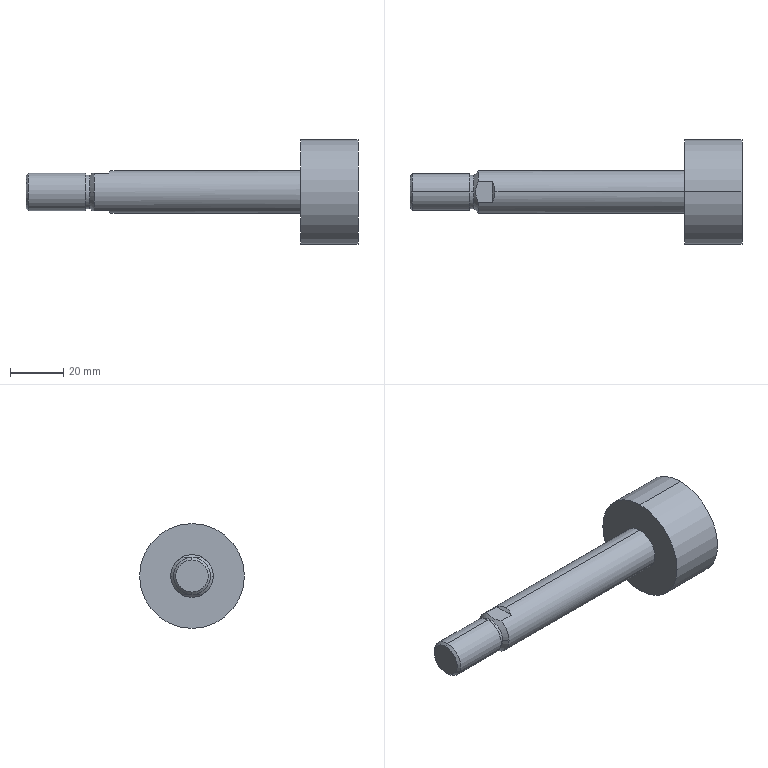Part | SolidWorks | features BaseBody 1 | 1 solid | 20 faces | box 125 x 39.5 x 39.5 mm | volume 45935 mm3 | cylinder 8 | plane 8 | cone 4 | commonest cylinder face diameters 12.6 x2 14 x2 16 x2 39.5 x2
STEP:
#1=CARTESIAN_POINT('',(-19.,3.873,7.));
#2=VERTEX_POINT('',#1);
#3=CARTESIAN_POINT('',(-18.,0.,8.));
#4=VERTEX_POINT('',#3);
#5=CARTESIAN_POINT('',(-19.,3.873,7.));
#6=CARTESIAN_POINT('',(-18.341,2.681,7.659));
#7=CARTESIAN_POINT('',(-18.,1.362,8.));
#8=CARTESIAN_POINT('',(-18.,0.,8.));
#9=(BOUNDED_CURVE()B_SPLINE_CURVE(3,(#5,#6,#7,#8),.UNSPECIFIED.,.F.,.F.)B_SPLINE_CURVE_WITH_KNOTS((4,4),(5.778,6.283),.UNSPECIFIED.)CURVE()GEOMETRIC_REPRESENTATION_ITEM()RATIONAL_B_SPLINE_CURVE((1.,0.9788,0.9788,1.))REPRESENTATION_ITEM(''));
#10=EDGE_CURVE('',#2,#4,#9,.T.);
#11=ORIENTED_EDGE('',*,*,#10,.T.);
#12=CARTESIAN_POINT('',(53.4,0.,8.));
#13=VERTEX_POINT('',#12);
#14=CARTESIAN_POINT('',(75.,0.,8.));
#15=DIRECTION('',(1.,0.,0.));
#16=VECTOR('',#15,1000.);
#17=LINE('',#14,#16);
#18=EDGE_CURVE('',#4,#13,#17,.T.);
#19=ORIENTED_EDGE('',*,*,#18,.T.);
#20=CARTESIAN_POINT('',(53.4,0.,-8.));
#21=VERTEX_POINT('',#20);
#22=CARTESIAN_POINT('',(53.4,0.,0.));
#23=DIRECTION('',(-1.,0.,0.));
#24=DIRECTION('',(0.,0.,-1.));
#25=AXIS2_PLACEMENT_3D('',#22,#23,#24);
#26=CIRCLE('',#25,8.);
#27=EDGE_CURVE('',#13,#21,#26,.T.);
#28=ORIENTED_EDGE('',*,*,#27,.T.);
#29=CARTESIAN_POINT('',(-18.,0.,-8.));
#30=VERTEX_POINT('',#29);
#31=CARTESIAN_POINT('',(75.,0.,-8.));
#32=DIRECTION('',(1.,0.,0.));
#33=VECTOR('',#32,1000.);
#34=LINE('',#31,#33);
#35=EDGE_CURVE('',#30,#21,#34,.T.);
#36=ORIENTED_EDGE('',*,*,#35,.F.);
#37=CARTESIAN_POINT('',(-19.,3.873,-7.));
#38=VERTEX_POINT('',#37);
#39=CARTESIAN_POINT('',(-18.,0.,-8.));
#40=CARTESIAN_POINT('',(-18.,1.362,-8.));
#41=CARTESIAN_POINT('',(-18.341,2.681,-7.659));
#42=CARTESIAN_POINT('',(-19.,3.873,-7.));
#43=(BOUNDED_CURVE()B_SPLINE_CURVE(3,(#39,#40,#41,#42),.UNSPECIFIED.,.F.,.F.)B_SPLINE_CURVE_WITH_KNOTS((4,4),(0.,0.5054),.UNSPECIFIED.)CURVE()GEOMETRIC_REPRESENTATION_ITEM()RATIONAL_B_SPLINE_CURVE((1.,0.9788,0.9788,1.))REPRESENTATION_ITEM(''));
#44=EDGE_CURVE('',#30,#38,#43,.T.);
#45=ORIENTED_EDGE('',*,*,#44,.T.);
#46=CARTESIAN_POINT('',(-24.3,3.873,-7.));
#47=VERTEX_POINT('',#46);
#48=CARTESIAN_POINT('',(75.,3.873,-7.));
#49=DIRECTION('',(-1.,0.,0.));
#50=VECTOR('',#49,1000.);
#51=LINE('',#48,#50);
#52=EDGE_CURVE('',#38,#47,#51,.T.);
#53=ORIENTED_EDGE('',*,*,#52,.T.);
#54=CARTESIAN_POINT('',(-24.3,8.,0.));
#55=VERTEX_POINT('',#54);
#56=CARTESIAN_POINT('',(-24.3,0.,0.));
#57=DIRECTION('',(1.,0.,0.));
#58=DIRECTION('',(0.,0.,-1.));
#59=AXIS2_PLACEMENT_3D('',#56,#57,#58);
#60=CIRCLE('',#59,8.);
#61=EDGE_CURVE('',#47,#55,#60,.T.);
#62=ORIENTED_EDGE('',*,*,#61,.T.);
#63=CARTESIAN_POINT('',(-24.3,3.873,7.));
#64=VERTEX_POINT('',#63);
#65=CARTESIAN_POINT('',(-24.3,0.,0.));
#66=DIRECTION('',(1.,0.,0.));
#67=DIRECTION('',(0.,0.,-1.));
#68=AXIS2_PLACEMENT_3D('',#65,#66,#67);
#69=CIRCLE('',#68,8.);
#70=EDGE_CURVE('',#55,#64,#69,.T.);
#71=ORIENTED_EDGE('',*,*,#70,.T.);
#72=CARTESIAN_POINT('',(75.,3.873,7.));
#73=DIRECTION('',(1.,0.,0.));
#74=VECTOR('',#73,1000.);
#75=LINE('',#72,#74);
#76=EDGE_CURVE('',#64,#2,#75,.T.);
#77=ORIENTED_EDGE('',*,*,#76,.T.);
#78=EDGE_LOOP('',(#11,#19,#28,#36,#45,#53,#62,#71,#77));
#79=FACE_OUTER_BOUND('',#78,.T.);
#80=CARTESIAN_POINT('',(75.,0.,0.));
#81=DIRECTION('',(1.,0.,0.));
#82=DIRECTION('',(0.,0.,-1.));
#83=AXIS2_PLACEMENT_3D('',#80,#81,#82);
#84=CYLINDRICAL_SURFACE('',#83,8.);
#85=ADVANCED_FACE('',(#79),#84,.T.);
#86=CARTESIAN_POINT('',(-26.,0.,6.3));
#87=VERTEX_POINT('',#86);
#88=CARTESIAN_POINT('',(-26.,-6.3,0.));
#89=VERTEX_POINT('',#88);
#90=CARTESIAN_POINT('',(-26.,0.,0.));
#91=DIRECTION('',(1.,0.,0.));
#92=DIRECTION('',(0.,0.,-1.));
#93=AXIS2_PLACEMENT_3D('',#90,#91,#92);
#94=CIRCLE('',#93,6.3);
#95=EDGE_CURVE('',#87,#89,#94,.T.);
#96=ORIENTED_EDGE('',*,*,#95,.T.);
#97=CARTESIAN_POINT('',(-24.3,-8.,0.));
#98=VERTEX_POINT('',#97);
#99=CARTESIAN_POINT('',(-24.3,-8.,0.));
#100=DIRECTION('',(0.7071,-0.7071,0.));
#101=VECTOR('',#100,1000.);
#102=LINE('',#99,#101);
#103=EDGE_CURVE('',#89,#98,#102,.T.);
#104=ORIENTED_EDGE('',*,*,#103,.T.);
#105=CARTESIAN_POINT('',(-24.3,-3.873,7.));
#106=VERTEX_POINT('',#105);
#107=CARTESIAN_POINT('',(-24.3,0.,0.));
#108=DIRECTION('',(1.,0.,0.));
#109=DIRECTION('',(0.,0.,-1.));
#110=AXIS2_PLACEMENT_3D('',#107,#108,#109);
#111=CIRCLE('',#110,8.);
#112=EDGE_CURVE('',#106,#98,#111,.T.);
#113=ORIENTED_EDGE('',*,*,#112,.F.);
#114=CARTESIAN_POINT('',(-24.3,3.873,7.));
#115=CARTESIAN_POINT('',(-24.594,3.265,7.));
#116=CARTESIAN_POINT('',(-24.843,2.645,7.));
#117=CARTESIAN_POINT('',(-25.107,1.682,7.));
#118=CARTESIAN_POINT('',(-25.177,1.356,7.));
#119=CARTESIAN_POINT('',(-25.274,0.6915,7.));
#120=CARTESIAN_POINT('',(-25.299,0.3497,7.));
#121=CARTESIAN_POINT('',(-25.301,-0.6617,7.));
#122=CARTESIAN_POINT('',(-25.204,-1.325,7.));
#123=CARTESIAN_POINT('',(-24.937,-2.305,7.));
#124=CARTESIAN_POINT('',(-24.829,-2.627,7.));
#125=CARTESIAN_POINT('',(-24.584,-3.258,7.));
#126=CARTESIAN_POINT('',(-24.448,-3.568,7.));
#127=CARTESIAN_POINT('',(-24.3,-3.873,7.));
#128=B_SPLINE_CURVE_WITH_KNOTS('',3,(#114,#115,#116,#117,#118,#119,#120,#121,#122,#123,#124,#125,#126,#127),.UNSPECIFIED.,.F.,.F.,(4,2,2,2,2,2,4),(0.,0.001996,0.002994,0.003992,0.005988,0.006986,0.007984),.UNSPECIFIED.);
#129=EDGE_CURVE('',#64,#106,#128,.T.);
#130=ORIENTED_EDGE('',*,*,#129,.F.);
#131=ORIENTED_EDGE('',*,*,#70,.F.);
#132=CARTESIAN_POINT('',(-26.,6.3,0.));
#133=VERTEX_POINT('',#132);
#134=CARTESIAN_POINT('',(-24.3,8.,0.));
#135=DIRECTION('',(0.7071,0.7071,0.));
#136=VECTOR('',#135,1000.);
#137=LINE('',#134,#136);
#138=EDGE_CURVE('',#133,#55,#137,.T.);
#139=ORIENTED_EDGE('',*,*,#138,.F.);
#140=CARTESIAN_POINT('',(-26.,0.,0.));
#141=DIRECTION('',(1.,0.,0.));
#142=DIRECTION('',(0.,0.,-1.));
#143=AXIS2_PLACEMENT_3D('',#140,#141,#142);
#144=CIRCLE('',#143,6.3);
#145=EDGE_CURVE('',#133,#87,#144,.T.);
#146=ORIENTED_EDGE('',*,*,#145,.T.);
#147=EDGE_LOOP('',(#96,#104,#113,#130,#131,#139,#146));
#148=FACE_OUTER_BOUND('',#147,.T.);
#149=CARTESIAN_POINT('',(-24.3,0.,0.));
#150=DIRECTION('',(1.,0.,0.));
#151=DIRECTION('',(0.,1.,0.));
#152=AXIS2_PLACEMENT_3D('',#149,#150,#151);
#153=CONICAL_SURFACE('',#152,8.,0.7854);
#154=ADVANCED_FACE('',(#148),#153,.T.);
#155=CARTESIAN_POINT('',(-27.5,0.,-6.3));
#156=VERTEX_POINT('',#155);
#157=CARTESIAN_POINT('',(-27.5,0.,6.3));
#158=VERTEX_POINT('',#157);
#159=CARTESIAN_POINT('',(-27.5,0.,0.));
#160=DIRECTION('',(1.,0.,0.));
#161=DIRECTION('',(0.,0.,-1.));
#162=AXIS2_PLACEMENT_3D('',#159,#160,#161);
#163=CIRCLE('',#162,6.3);
#164=EDGE_CURVE('',#156,#158,#163,.T.);
#165=ORIENTED_EDGE('',*,*,#164,.T.);
#166=CARTESIAN_POINT('',(75.,0.,6.3));
#167=DIRECTION('',(1.,0.,0.));
#168=VECTOR('',#167,1000.);
#169=LINE('',#166,#168);
#170=EDGE_CURVE('',#158,#87,#169,.T.);
#171=ORIENTED_EDGE('',*,*,#170,.T.);
#172=ORIENTED_EDGE('',*,*,#145,.F.);
#173=CARTESIAN_POINT('',(-26.,0.,-6.3));
#174=VERTEX_POINT('',#173);
#175=CARTESIAN_POINT('',(-26.,0.,0.));
#176=DIRECTION('',(1.,0.,0.));
#177=DIRECTION('',(0.,0.,-1.));
#178=AXIS2_PLACEMENT_3D('',#175,#176,#177);
#179=CIRCLE('',#178,6.3);
#180=EDGE_CURVE('',#174,#133,#179,.T.);
#181=ORIENTED_EDGE('',*,*,#180,.F.);
#182=CARTESIAN_POINT('',(75.,0.,-6.3));
#183=DIRECTION('',(1.,0.,0.));
#184=VECTOR('',#183,1000.);
#185=LINE('',#182,#184);
#186=EDGE_CURVE('',#156,#174,#185,.T.);
#187=ORIENTED_EDGE('',*,*,#186,.F.);
#188=EDGE_LOOP('',(#165,#171,#172,#181,#187));
#189=FACE_OUTER_BOUND('',#188,.T.);
#190=CARTESIAN_POINT('',(75.,0.,0.));
#191=DIRECTION('',(1.,0.,0.));
#192=DIRECTION('',(0.,0.,-1.));
#193=AXIS2_PLACEMENT_3D('',#190,#191,#192);
#194=CYLINDRICAL_SURFACE('',#193,6.3);
#195=ADVANCED_FACE('',(#189),#194,.T.);
#196=CARTESIAN_POINT('',(53.4,0.,-19.75));
#197=VERTEX_POINT('',#196);
#198=CARTESIAN_POINT('',(53.4,0.,19.75));
#199=VERTEX_POINT('',#198);
#200=CARTESIAN_POINT('',(53.4,0.,0.));
#201=DIRECTION('',(1.,0.,0.));
#202=DIRECTION('',(0.,0.,-1.));
#203=AXIS2_PLACEMENT_3D('',#200,#201,#202);
#204=CIRCLE('',#203,19.75);
#205=EDGE_CURVE('',#197,#199,#204,.T.);
#206=ORIENTED_EDGE('',*,*,#205,.T.);
#207=CARTESIAN_POINT('',(75.,0.,19.75));
#208=VERTEX_POINT('',#207);
#209=CARTESIAN_POINT('',(75.,0.,19.75));
#210=DIRECTION('',(1.,0.,0.));
#211=VECTOR('',#210,1000.);
#212=LINE('',#209,#211);
#213=EDGE_CURVE('',#199,#208,#212,.T.);
#214=ORIENTED_EDGE('',*,*,#213,.T.);
#215=CARTESIAN_POINT('',(75.,0.,-19.75));
#216=VERTEX_POINT('',#215);
#217=CARTESIAN_POINT('',(75.,0.,0.));
#218=DIRECTION('',(-1.,0.,0.));
#219=DIRECTION('',(0.,0.,-1.));
#220=AXIS2_PLACEMENT_3D('',#217,#218,#219);
#221=CIRCLE('',#220,19.75);
#222=EDGE_CURVE('',#208,#216,#221,.T.);
#223=ORIENTED_EDGE('',*,*,#222,.T.);
#224=CARTESIAN_POINT('',(75.,0.,-19.75));
#225=DIRECTION('',(1.,0.,0.));
#226=VECTOR('',#225,1000.);
#227=LINE('',#224,#226);
#228=EDGE_CURVE('',#197,#216,#227,.T.);
#229=ORIENTED_EDGE('',*,*,#228,.F.);
#230=EDGE_LOOP('',(#206,#214,#223,#229));
#231=FACE_OUTER_BOUND('',#230,.T.);
#232=CARTESIAN_POINT('',(75.,0.,0.));
#233=DIRECTION('',(1.,0.,0.));
#234=DIRECTION('',(0.,0.,-1.));
#235=AXIS2_PLACEMENT_3D('',#232,#233,#234);
#236=CYLINDRICAL_SURFACE('',#235,19.75);
#237=ADVANCED_FACE('',(#231),#236,.T.);
#238=CARTESIAN_POINT('',(-49.08,0.,-7.));
#239=VERTEX_POINT('',#238);
#240=CARTESIAN_POINT('',(-49.08,0.,7.));
#241=VERTEX_POINT('',#240);
#242=CARTESIAN_POINT('',(-49.08,0.,0.));
#243=DIRECTION('',(1.,0.,0.));
#244=DIRECTION('',(0.,0.,-1.));
#245=AXIS2_PLACEMENT_3D('',#242,#243,#244);
#246=CIRCLE('',#245,7.);
#247=EDGE_CURVE('',#239,#241,#246,.T.);
#248=ORIENTED_EDGE('',*,*,#247,.T.);
#249=CARTESIAN_POINT('',(-27.5,0.,7.));
#250=VERTEX_POINT('',#249);
#251=CARTESIAN_POINT('',(75.,0.,7.));
#252=DIRECTION('',(1.,0.,0.));
#253=VECTOR('',#252,1000.);
#254=LINE('',#251,#253);
#255=EDGE_CURVE('',#241,#250,#254,.T.);
#256=ORIENTED_EDGE('',*,*,#255,.T.);
#257=CARTESIAN_POINT('',(-27.5,0.,-7.));
#258=VERTEX_POINT('',#257);
#259=CARTESIAN_POINT('',(-27.5,0.,0.));
#260=DIRECTION('',(-1.,0.,0.));
#261=DIRECTION('',(0.,0.,-1.));
#262=AXIS2_PLACEMENT_3D('',#259,#260,#261);
#263=CIRCLE('',#262,7.);
#264=EDGE_CURVE('',#250,#258,#263,.T.);
#265=ORIENTED_EDGE('',*,*,#264,.T.);
#266=CARTESIAN_POINT('',(75.,0.,-7.));
#267=DIRECTION('',(1.,0.,0.));
#268=VECTOR('',#267,1000.);
#269=LINE('',#266,#268);
#270=EDGE_CURVE('',#239,#258,#269,.T.);
#271=ORIENTED_EDGE('',*,*,#270,.F.);
#272=EDGE_LOOP('',(#248,#256,#265,#271));
#273=FACE_OUTER_BOUND('',#272,.T.);
#274=CARTESIAN_POINT('',(75.,0.,0.));
#275=DIRECTION('',(1.,0.,0.));
#276=DIRECTION('',(0.,0.,-1.));
#277=AXIS2_PLACEMENT_3D('',#274,#275,#276);
#278=CYLINDRICAL_SURFACE('',#277,7.);
#279=ADVANCED_FACE('',(#273),#278,.T.);
#280=CARTESIAN_POINT('',(-50.,0.,-6.08));
#281=VERTEX_POINT('',#280);
#282=CARTESIAN_POINT('',(-50.,0.,6.08));
#283=VERTEX_POINT('',#282);
#284=CARTESIAN_POINT('',(-50.,0.,0.));
#285=DIRECTION('',(1.,0.,0.));
#286=DIRECTION('',(0.,0.,-1.));
#287=AXIS2_PLACEMENT_3D('',#284,#285,#286);
#288=CIRCLE('',#287,6.08);
#289=EDGE_CURVE('',#281,#283,#288,.T.);
#290=ORIENTED_EDGE('',*,*,#289,.T.);
#291=CARTESIAN_POINT('',(-49.08,0.,7.));
#292=DIRECTION('',(0.7071,0.,0.7071));
#293=VECTOR('',#292,1000.);
#294=LINE('',#291,#293);
#295=EDGE_CURVE('',#283,#241,#294,.T.);
#296=ORIENTED_EDGE('',*,*,#295,.T.);
#297=ORIENTED_EDGE('',*,*,#247,.F.);
#298=CARTESIAN_POINT('',(-49.08,0.,-7.));
#299=DIRECTION('',(0.7071,0.,-0.7071));
#300=VECTOR('',#299,1000.);
#301=LINE('',#298,#300);
#302=EDGE_CURVE('',#281,#239,#301,.T.);
#303=ORIENTED_EDGE('',*,*,#302,.F.);
#304=EDGE_LOOP('',(#290,#296,#297,#303));
#305=FACE_OUTER_BOUND('',#304,.T.);
#306=CARTESIAN_POINT('',(-49.08,0.,0.));
#307=DIRECTION('',(1.,0.,0.));
#308=DIRECTION('',(0.,0.,-1.));
#309=AXIS2_PLACEMENT_3D('',#306,#307,#308);
#310=CONICAL_SURFACE('',#309,7.,0.7854);
#311=ADVANCED_FACE('',(#305),#310,.T.);
#312=ORIENTED_EDGE('',*,*,#18,.F.);
#313=CARTESIAN_POINT('',(-19.,-3.873,7.));
#314=VERTEX_POINT('',#313);
#315=CARTESIAN_POINT('',(-18.,0.,8.));
#316=CARTESIAN_POINT('',(-18.,-1.362,8.));
#317=CARTESIAN_POINT('',(-18.341,-2.681,7.659));
#318=CARTESIAN_POINT('',(-19.,-3.873,7.));
#319=(BOUNDED_CURVE()B_SPLINE_CURVE(3,(#315,#316,#317,#318),.UNSPECIFIED.,.F.,.F.)B_SPLINE_CURVE_WITH_KNOTS((4,4),(0.,0.5054),.UNSPECIFIED.)CURVE()GEOMETRIC_REPRESENTATION_ITEM()RATIONAL_B_SPLINE_CURVE((1.,0.9788,0.9788,1.))REPRESENTATION_ITEM(''));
#320=EDGE_CURVE('',#4,#314,#319,.T.);
#321=ORIENTED_EDGE('',*,*,#320,.T.);
#322=CARTESIAN_POINT('',(75.,-3.873,7.));
#323=DIRECTION('',(-1.,0.,0.));
#324=VECTOR('',#323,1000.);
#325=LINE('',#322,#324);
#326=EDGE_CURVE('',#314,#106,#325,.T.);
#327=ORIENTED_EDGE('',*,*,#326,.T.);
#328=ORIENTED_EDGE('',*,*,#112,.T.);
#329=CARTESIAN_POINT('',(-24.3,-3.873,-7.));
#330=VERTEX_POINT('',#329);
#331=CARTESIAN_POINT('',(-24.3,0.,0.));
#332=DIRECTION('',(1.,0.,0.));
#333=DIRECTION('',(0.,0.,-1.));
#334=AXIS2_PLACEMENT_3D('',#331,#332,#333);
#335=CIRCLE('',#334,8.);
#336=EDGE_CURVE('',#98,#330,#335,.T.);
#337=ORIENTED_EDGE('',*,*,#336,.T.);
#338=CARTESIAN_POINT('',(-19.,-3.873,-7.));
#339=VERTEX_POINT('',#338);
#340=CARTESIAN_POINT('',(75.,-3.873,-7.));
#341=DIRECTION('',(1.,0.,0.));
#342=VECTOR('',#341,1000.);
#343=LINE('',#340,#342);
#344=EDGE_CURVE('',#330,#339,#343,.T.);
#345=ORIENTED_EDGE('',*,*,#344,.T.);
#346=CARTESIAN_POINT('',(-19.,-3.873,-7.));
#347=CARTESIAN_POINT('',(-18.341,-2.681,-7.659));
#348=CARTESIAN_POINT('',(-18.,-1.362,-8.));
#349=CARTESIAN_POINT('',(-18.,0.,-8.));
#350=(BOUNDED_CURVE()B_SPLINE_CURVE(3,(#346,#347,#348,#349),.UNSPECIFIED.,.F.,.T.)B_SPLINE_CURVE_WITH_KNOTS((4,4),(5.778,6.283),.UNSPECIFIED.)CURVE()GEOMETRIC_REPRESENTATION_ITEM()RATIONAL_B_SPLINE_CURVE((1.,0.9788,0.9788,1.))REPRESENTATION_ITEM(''));
#351=EDGE_CURVE('',#339,#30,#350,.T.);
#352=ORIENTED_EDGE('',*,*,#351,.T.);
#353=ORIENTED_EDGE('',*,*,#35,.T.);
#354=CARTESIAN_POINT('',(53.4,0.,0.));
#355=DIRECTION('',(-1.,0.,0.));
#356=DIRECTION('',(0.,0.,-1.));
#357=AXIS2_PLACEMENT_3D('',#354,#355,#356);
#358=CIRCLE('',#357,8.);
#359=EDGE_CURVE('',#21,#13,#358,.T.);
#360=ORIENTED_EDGE('',*,*,#359,.T.);
#361=EDGE_LOOP('',(#312,#321,#327,#328,#337,#345,#352,#353,#360));
#362=FACE_OUTER_BOUND('',#361,.T.);
#363=CARTESIAN_POINT('',(75.,0.,0.));
#364=DIRECTION('',(1.,0.,0.));
#365=DIRECTION('',(0.,0.,-1.));
#366=AXIS2_PLACEMENT_3D('',#363,#364,#365);
#367=CYLINDRICAL_SURFACE('',#366,8.);
#368=ADVANCED_FACE('',(#362),#367,.T.);
#369=ORIENTED_EDGE('',*,*,#10,.F.);
#370=CARTESIAN_POINT('',(-19.,8.,7.));
#371=DIRECTION('',(0.,-1.,0.));
#372=VECTOR('',#371,1000.);
#373=LINE('',#370,#372);
#374=EDGE_CURVE('',#2,#314,#373,.T.);
#375=ORIENTED_EDGE('',*,*,#374,.T.);
#376=ORIENTED_EDGE('',*,*,#320,.F.);
#377=EDGE_LOOP('',(#369,#375,#376));
#378=FACE_OUTER_BOUND('',#377,.T.);
#379=CARTESIAN_POINT('',(-2.,8.,24.));
#380=DIRECTION('',(-0.7071,0.,0.7071));
#381=DIRECTION('',(0.7071,0.,0.7071));
#382=AXIS2_PLACEMENT_3D('',#379,#380,#381);
#383=PLANE('',#382);
#384=ADVANCED_FACE('',(#378),#383,.T.);
#385=ORIENTED_EDGE('',*,*,#76,.F.);
#386=ORIENTED_EDGE('',*,*,#129,.T.);
#387=ORIENTED_EDGE('',*,*,#326,.F.);
#388=ORIENTED_EDGE('',*,*,#374,.F.);
#389=EDGE_LOOP('',(#385,#386,#387,#388));
#390=FACE_OUTER_BOUND('',#389,.T.);
#391=CARTESIAN_POINT('',(-19.,8.,7.));
#392=DIRECTION('',(0.,0.,1.));
#393=DIRECTION('',(1.,0.,0.));
#394=AXIS2_PLACEMENT_3D('',#391,#392,#393);
#395=PLANE('',#394);
#396=ADVANCED_FACE('',(#390),#395,.T.);
#397=ORIENTED_EDGE('',*,*,#103,.F.);
#398=CARTESIAN_POINT('',(-26.,0.,0.));
#399=DIRECTION('',(1.,0.,0.));
#400=DIRECTION('',(0.,0.,-1.));
#401=AXIS2_PLACEMENT_3D('',#398,#399,#400);
#402=CIRCLE('',#401,6.3);
#403=EDGE_CURVE('',#89,#174,#402,.T.);
#404=ORIENTED_EDGE('',*,*,#403,.T.);
#405=ORIENTED_EDGE('',*,*,#180,.T.);
#406=ORIENTED_EDGE('',*,*,#138,.T.);
#407=ORIENTED_EDGE('',*,*,#61,.F.);
#408=CARTESIAN_POINT('',(-24.3,3.873,-7.));
#409=CARTESIAN_POINT('',(-24.594,3.265,-7.));
#410=CARTESIAN_POINT('',(-24.843,2.645,-7.));
#411=CARTESIAN_POINT('',(-25.107,1.682,-7.));
#412=CARTESIAN_POINT('',(-25.177,1.356,-7.));
#413=CARTESIAN_POINT('',(-25.274,0.6915,-7.));
#414=CARTESIAN_POINT('',(-25.299,0.3497,-7.));
#415=CARTESIAN_POINT('',(-25.301,-0.6617,-7.));
#416=CARTESIAN_POINT('',(-25.204,-1.325,-7.));
#417=CARTESIAN_POINT('',(-24.937,-2.305,-7.));
#418=CARTESIAN_POINT('',(-24.829,-2.627,-7.));
#419=CARTESIAN_POINT('',(-24.584,-3.258,-7.));
#420=CARTESIAN_POINT('',(-24.448,-3.568,-7.));
#421=CARTESIAN_POINT('',(-24.3,-3.873,-7.));
#422=B_SPLINE_CURVE_WITH_KNOTS('',3,(#408,#409,#410,#411,#412,#413,#414,#415,#416,#417,#418,#419,#420,#421),.UNSPECIFIED.,.F.,.F.,(4,2,2,2,2,2,4),(0.,0.001996,0.002994,0.003992,0.005988,0.006986,0.007984),.UNSPECIFIED.);
#423=EDGE_CURVE('',#47,#330,#422,.T.);
#424=ORIENTED_EDGE('',*,*,#423,.T.);
#425=ORIENTED_EDGE('',*,*,#336,.F.);
#426=EDGE_LOOP('',(#397,#404,#405,#406,#407,#424,#425));
#427=FACE_OUTER_BOUND('',#426,.T.);
#428=CARTESIAN_POINT('',(-24.3,0.,0.));
#429=DIRECTION('',(1.,0.,0.));
#430=DIRECTION('',(0.,1.,0.));
#431=AXIS2_PLACEMENT_3D('',#428,#429,#430);
#432=CONICAL_SURFACE('',#431,8.,0.7854);
#433=ADVANCED_FACE('',(#427),#432,.T.);
#434=ORIENTED_EDGE('',*,*,#344,.F.);
#435=ORIENTED_EDGE('',*,*,#423,.F.);
#436=ORIENTED_EDGE('',*,*,#52,.F.);
#437=CARTESIAN_POINT('',(-19.,8.,-7.));
#438=DIRECTION('',(0.,-1.,0.));
#439=VECTOR('',#438,1000.);
#440=LINE('',#437,#439);
#441=EDGE_CURVE('',#38,#339,#440,.T.);
#442=ORIENTED_EDGE('',*,*,#441,.T.);
#443=EDGE_LOOP('',(#434,#435,#436,#442));
#444=FACE_OUTER_BOUND('',#443,.T.);
#445=CARTESIAN_POINT('',(-26.,8.,-7.));
#446=DIRECTION('',(0.,0.,-1.));
#447=DIRECTION('',(-1.,0.,0.));
#448=AXIS2_PLACEMENT_3D('',#445,#446,#447);
#449=PLANE('',#448);
#450=ADVANCED_FACE('',(#444),#449,.T.);
#451=ORIENTED_EDGE('',*,*,#351,.F.);
#452=ORIENTED_EDGE('',*,*,#441,.F.);
#453=ORIENTED_EDGE('',*,*,#44,.F.);
#454=EDGE_LOOP('',(#451,#452,#453));
#455=FACE_OUTER_BOUND('',#454,.T.);
#456=CARTESIAN_POINT('',(-19.,8.,-7.));
#457=DIRECTION('',(-0.7071,0.,-0.7071));
#458=DIRECTION('',(-0.7071,0.,0.7071));
#459=AXIS2_PLACEMENT_3D('',#456,#457,#458);
#460=PLANE('',#459);
#461=ADVANCED_FACE('',(#455),#460,.T.);
#462=ORIENTED_EDGE('',*,*,#359,.F.);
#463=ORIENTED_EDGE('',*,*,#27,.F.);
#464=EDGE_LOOP('',(#462,#463));
#465=FACE_BOUND('',#464,.T.);
#466=ORIENTED_EDGE('',*,*,#205,.F.);
#467=CARTESIAN_POINT('',(53.4,0.,0.));
#468=DIRECTION('',(1.,0.,0.));
#469=DIRECTION('',(0.,0.,-1.));
#470=AXIS2_PLACEMENT_3D('',#467,#468,#469);
#471=CIRCLE('',#470,19.75);
#472=EDGE_CURVE('',#199,#197,#471,.T.);
#473=ORIENTED_EDGE('',*,*,#472,.F.);
#474=EDGE_LOOP('',(#466,#473));
#475=FACE_OUTER_BOUND('',#474,.T.);
#476=CARTESIAN_POINT('',(53.4,8.,0.));
#477=DIRECTION('',(1.,0.,0.));
#478=DIRECTION('',(0.,0.,-1.));
#479=AXIS2_PLACEMENT_3D('',#476,#477,#478);
#480=PLANE('',#479);
#481=ADVANCED_FACE('',(#465,#475),#480,.F.);
#482=ORIENTED_EDGE('',*,*,#170,.F.);
#483=CARTESIAN_POINT('',(-27.5,0.,0.));
#484=DIRECTION('',(1.,0.,0.));
#485=DIRECTION('',(0.,0.,-1.));
#486=AXIS2_PLACEMENT_3D('',#483,#484,#485);
#487=CIRCLE('',#486,6.3);
#488=EDGE_CURVE('',#158,#156,#487,.T.);
#489=ORIENTED_EDGE('',*,*,#488,.T.);
#490=ORIENTED_EDGE('',*,*,#186,.T.);
#491=ORIENTED_EDGE('',*,*,#403,.F.);
#492=ORIENTED_EDGE('',*,*,#95,.F.);
#493=EDGE_LOOP('',(#482,#489,#490,#491,#492));
#494=FACE_OUTER_BOUND('',#493,.T.);
#495=CARTESIAN_POINT('',(75.,0.,0.));
#496=DIRECTION('',(1.,0.,0.));
#497=DIRECTION('',(0.,0.,-1.));
#498=AXIS2_PLACEMENT_3D('',#495,#496,#497);
#499=CYLINDRICAL_SURFACE('',#498,6.3);
#500=ADVANCED_FACE('',(#494),#499,.T.);
#501=ORIENTED_EDGE('',*,*,#213,.F.);
#502=ORIENTED_EDGE('',*,*,#472,.T.);
#503=ORIENTED_EDGE('',*,*,#228,.T.);
#504=CARTESIAN_POINT('',(75.,0.,0.));
#505=DIRECTION('',(-1.,0.,0.));
#506=DIRECTION('',(0.,0.,-1.));
#507=AXIS2_PLACEMENT_3D('',#504,#505,#506);
#508=CIRCLE('',#507,19.75);
#509=EDGE_CURVE('',#216,#208,#508,.T.);
#510=ORIENTED_EDGE('',*,*,#509,.T.);
#511=EDGE_LOOP('',(#501,#502,#503,#510));
#512=FACE_OUTER_BOUND('',#511,.T.);
#513=CARTESIAN_POINT('',(75.,0.,0.));
#514=DIRECTION('',(1.,0.,0.));
#515=DIRECTION('',(0.,0.,-1.));
#516=AXIS2_PLACEMENT_3D('',#513,#514,#515);
#517=CYLINDRICAL_SURFACE('',#516,19.75);
#518=ADVANCED_FACE('',(#512),#517,.T.);
#519=CARTESIAN_POINT('',(-27.5,0.,0.));
#520=DIRECTION('',(-1.,0.,0.));
#521=DIRECTION('',(0.,0.,-1.));
#522=AXIS2_PLACEMENT_3D('',#519,#520,#521);
#523=CIRCLE('',#522,7.);
#524=EDGE_CURVE('',#258,#250,#523,.T.);
#525=ORIENTED_EDGE('',*,*,#524,.F.);
#526=ORIENTED_EDGE('',*,*,#264,.F.);
#527=EDGE_LOOP('',(#525,#526));
#528=FACE_OUTER_BOUND('',#527,.T.);
#529=ORIENTED_EDGE('',*,*,#164,.F.);
#530=ORIENTED_EDGE('',*,*,#488,.F.);
#531=EDGE_LOOP('',(#529,#530));
#532=FACE_BOUND('',#531,.T.);
#533=CARTESIAN_POINT('',(-27.5,7.,0.));
#534=DIRECTION('',(-1.,0.,0.));
#535=DIRECTION('',(0.,0.,1.));
#536=AXIS2_PLACEMENT_3D('',#533,#534,#535);
#537=PLANE('',#536);
#538=ADVANCED_FACE('',(#528,#532),#537,.F.);
#539=ORIENTED_EDGE('',*,*,#509,.F.);
#540=ORIENTED_EDGE('',*,*,#222,.F.);
#541=EDGE_LOOP('',(#539,#540));
#542=FACE_OUTER_BOUND('',#541,.T.);
#543=CARTESIAN_POINT('',(75.,19.75,0.));
#544=DIRECTION('',(-1.,0.,0.));
#545=DIRECTION('',(0.,0.,1.));
#546=AXIS2_PLACEMENT_3D('',#543,#544,#545);
#547=PLANE('',#546);
#548=ADVANCED_FACE('',(#542),#547,.F.);
#549=ORIENTED_EDGE('',*,*,#255,.F.);
#550=CARTESIAN_POINT('',(-49.08,0.,0.));
#551=DIRECTION('',(1.,0.,0.));
#552=DIRECTION('',(0.,0.,-1.));
#553=AXIS2_PLACEMENT_3D('',#550,#551,#552);
#554=CIRCLE('',#553,7.);
#555=EDGE_CURVE('',#241,#239,#554,.T.);
#556=ORIENTED_EDGE('',*,*,#555,.T.);
#557=ORIENTED_EDGE('',*,*,#270,.T.);
#558=ORIENTED_EDGE('',*,*,#524,.T.);
#559=EDGE_LOOP('',(#549,#556,#557,#558));
#560=FACE_OUTER_BOUND('',#559,.T.);
#561=CARTESIAN_POINT('',(75.,0.,0.));
#562=DIRECTION('',(1.,0.,0.));
#563=DIRECTION('',(0.,0.,-1.));
#564=AXIS2_PLACEMENT_3D('',#561,#562,#563);
#565=CYLINDRICAL_SURFACE('',#564,7.);
#566=ADVANCED_FACE('',(#560),#565,.T.);
#567=ORIENTED_EDGE('',*,*,#295,.F.);
#568=CARTESIAN_POINT('',(-50.,0.,0.));
#569=DIRECTION('',(1.,0.,0.));
#570=DIRECTION('',(0.,0.,-1.));
#571=AXIS2_PLACEMENT_3D('',#568,#569,#570);
#572=CIRCLE('',#571,6.08);
#573=EDGE_CURVE('',#283,#281,#572,.T.);
#574=ORIENTED_EDGE('',*,*,#573,.T.);
#575=ORIENTED_EDGE('',*,*,#302,.T.);
#576=ORIENTED_EDGE('',*,*,#555,.F.);
#577=EDGE_LOOP('',(#567,#574,#575,#576));
#578=FACE_OUTER_BOUND('',#577,.T.);
#579=CARTESIAN_POINT('',(-49.08,0.,0.));
#580=DIRECTION('',(1.,0.,0.));
#581=DIRECTION('',(0.,0.,-1.));
#582=AXIS2_PLACEMENT_3D('',#579,#580,#581);
#583=CONICAL_SURFACE('',#582,7.,0.7854);
#584=ADVANCED_FACE('',(#578),#583,.T.);
#585=ORIENTED_EDGE('',*,*,#289,.F.);
#586=ORIENTED_EDGE('',*,*,#573,.F.);
#587=EDGE_LOOP('',(#585,#586));
#588=FACE_OUTER_BOUND('',#587,.T.);
#589=CARTESIAN_POINT('',(-50.,0.,0.));
#590=DIRECTION('',(1.,0.,0.));
#591=DIRECTION('',(0.,0.,-1.));
#592=AXIS2_PLACEMENT_3D('',#589,#590,#591);
#593=PLANE('',#592);
#594=ADVANCED_FACE('',(#588),#593,.F.);
#595=CLOSED_SHELL('',(#85,#154,#195,#237,#279,#311,#368,#384,#396,#433,#450,#461,#481,#500,#518,#538,#548,#566,#584,#594));
#596=MANIFOLD_SOLID_BREP('',#595);
#597=CARTESIAN_POINT('',(0.,0.,0.));
#598=DIRECTION('',(0.,0.,1.));
#599=DIRECTION('',(1.,0.,0.));
#600=AXIS2_PLACEMENT_3D('',#597,#598,#599);
#601=(LENGTH_UNIT()NAMED_UNIT(*)SI_UNIT(.MILLI.,.METRE.));
#602=UNCERTAINTY_MEASURE_WITH_UNIT(LENGTH_MEASURE(0.00001),#601,'','');
#603=(NAMED_UNIT(*)PLANE_ANGLE_UNIT()SI_UNIT($,.RADIAN.));
#604=(NAMED_UNIT(*)SI_UNIT($,.STERADIAN.)SOLID_ANGLE_UNIT());
#605=(GEOMETRIC_REPRESENTATION_CONTEXT(3)GLOBAL_UNCERTAINTY_ASSIGNED_CONTEXT((#602))GLOBAL_UNIT_ASSIGNED_CONTEXT((#601,#603,#604))REPRESENTATION_CONTEXT('',''));
#606=ADVANCED_BREP_SHAPE_REPRESENTATION('',(#596,#600),#605);